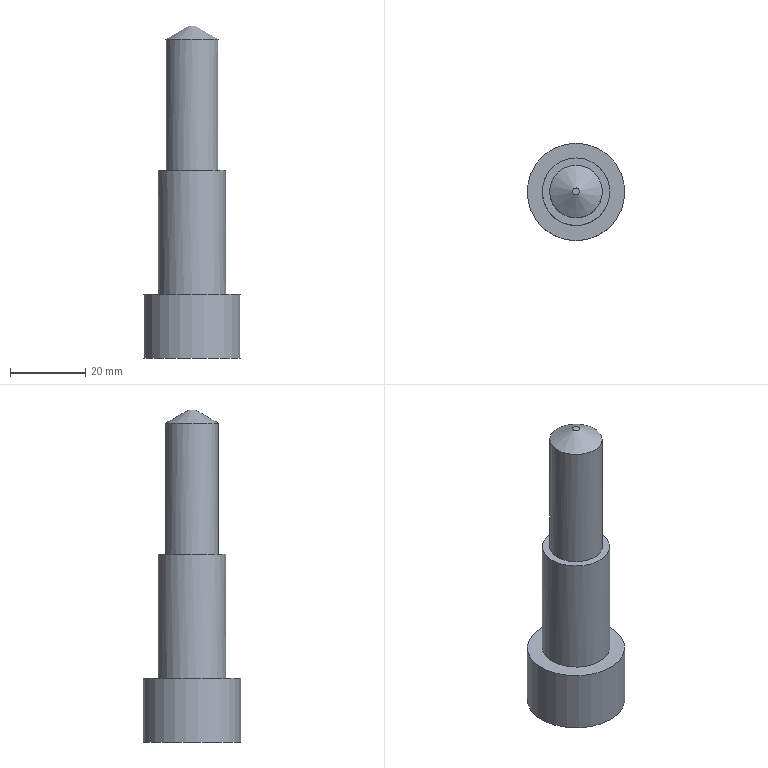Part | STEP file | solid 227 | 1 solid | 8 faces | box 26 x 26 x 88.5 mm | volume 23018 mm3 | plane 4 | cylinder 3 | cone 1 | commonest cylinder face diameters 14 x1 18 x1 26 x1